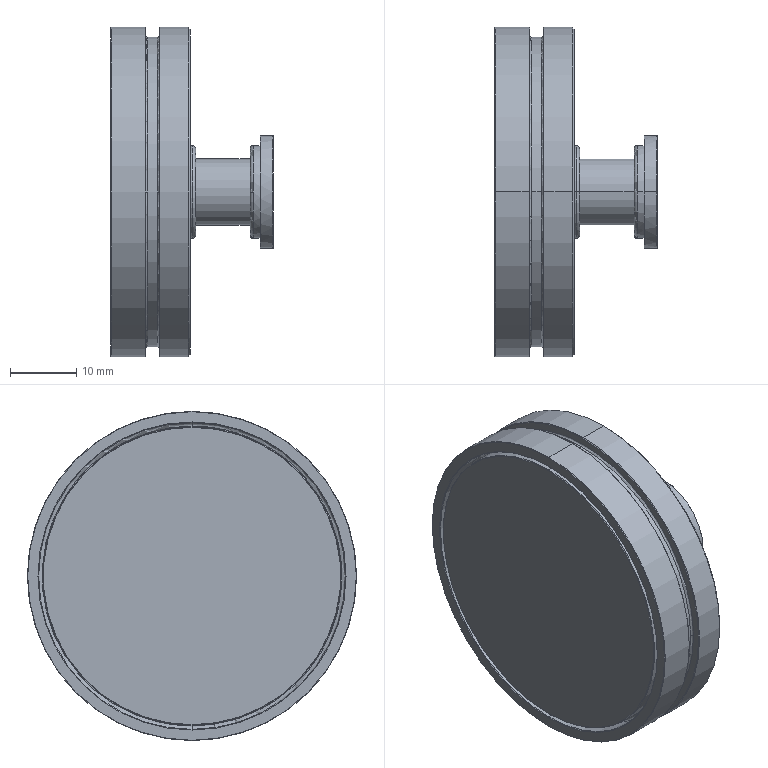Part | NX | features BREP 1 | 1 solid | 288 faces | box 24.5 x 49.6 x 49.6 mm | volume 18037 mm3 | cylinder 185 | cone 41 | plane 40 | torus 14 | spline 8 | commonest cylinder face diameters 3.3 x66 4.015 x66 7 x10 4 x8 17 x6 27 x5